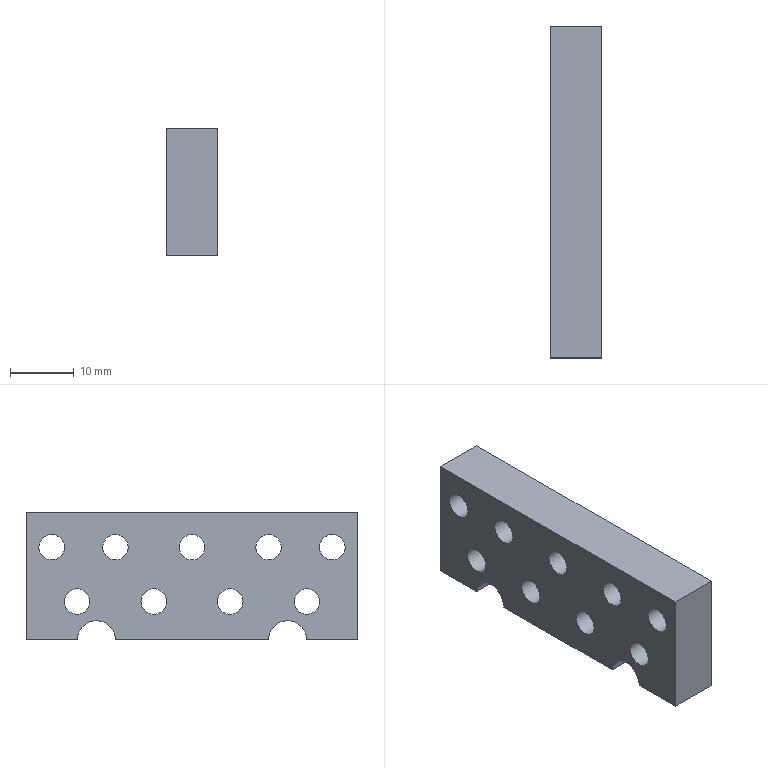Part | STEP file | 1-68.2 | 1 solid | 19 faces | box 8 x 52 x 20 mm | volume 7189 mm3 | cylinder 11 | plane 8 | commonest cylinder face diameters 4 x9 6 x2